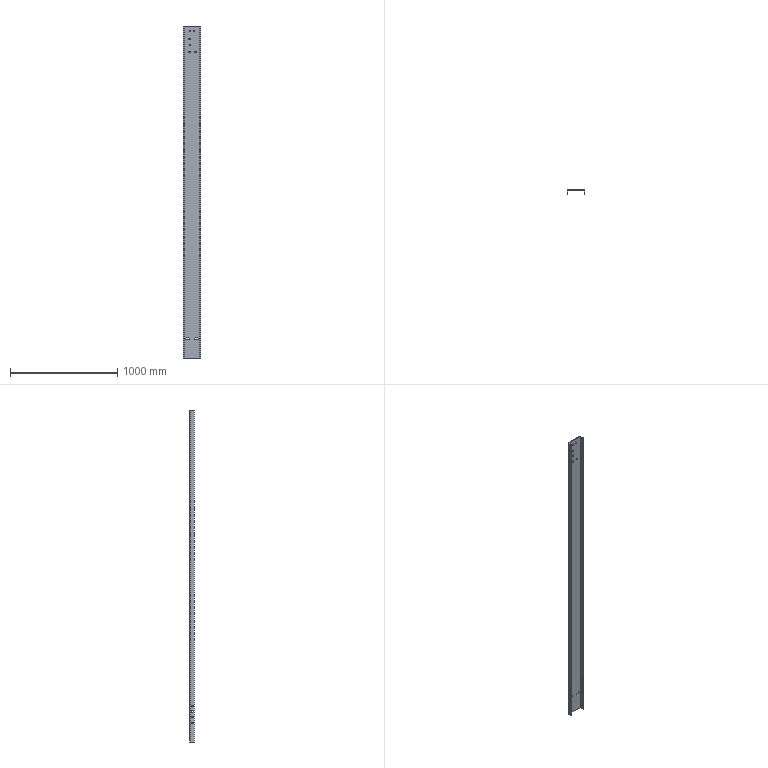Part | 1 solid | 84 faces | box 160 x 45 x 3100 mm | volume 3657117 mm3 | cylinder 46 | plane 38 | commonest cylinder face diameters 13 x32 12 x6 14 x6 2 x2